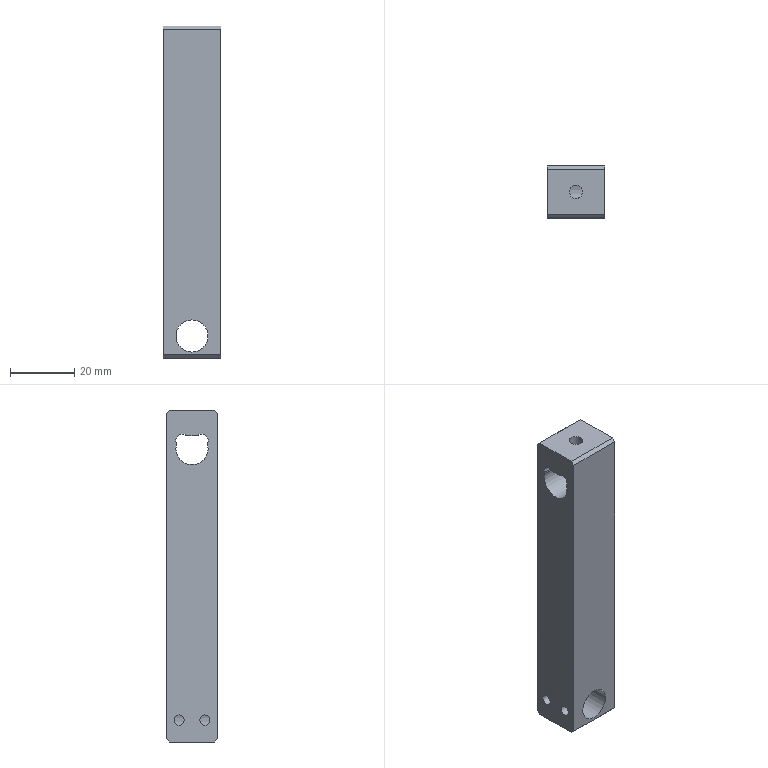NC program | NX | posted by the shop | part box 18 x 16 x 103.264 mm
Whole program:
%
O0001
(Machine time: 45.49 MIN)
(===Total Tool:6===)
(T2=D6 chamfer mill   D=6.   R=0.   D-  H02 Z=-2.15 )
(T13=ZT3.3  D=3.3  DR_a=118 D-  H13 Z=-10.  )
(T16=ZT6.8  D=6.8  DR_a=118 D-  H16 Z=-22.  )
(T4=D4      D=4.   R=0.   D-  H04 Z=-18.5 )
(T21=M4X0.7 D=3.3  DR_a=180 D-  H21 Z=-7.   )
(T11=D4-J   D=4.   R=0.   D11 H11 Z=-18.5 )
G80 G90 G17 G49 G40
G91 G28 Z0
M01
N1 T02 M06
(D6 chamfer mill  D=6. R=0. H=02 ce=0.00 di=0.00)
G00 G90 G54 X96.43 Y-12. M03 S8000
G43 H02 Z20.
M08
G98 G81 X96.43 Y-12. Z-.8 R1. F500.
Y-4.
G80
G00 Z20.
G00 G90 X12. Y-8. M03 S8000
Z20.
G98 G81 X12. Y-8. Z-.8 R1. F500.
G80
G00 Z20.
G91 G28 Z0.0
M05
M09
G91 G28 Z0.0
M01
N2 T13 M06
(ZT3.3 D=3.3 DR_a=118 H=13)
G00 G90 G54 X96.43 Y-12. M03 S3000
G43 H13 Z20.
M08
G98 G83 X96.43 Y-12. Z-10. R1. F300. Q2.
Y-4.
G80
G00 Z20.
G91 G28 Z0.0
M05
M09
G91 G28 Z0.0
M01
N3 T16 M06
(ZT6.8 D=6.8 DR_a=118 H=16)
G00 G90 G54 X12. Y-8. M03 S2000
G43 H16 Z20.
M08
G98 G83 X12. Y-8. Z-22. R1. F300. Q2.
G80
G00 Z20.
G91 G28 Z0.0
M05
M09
G91 G28 Z0.0
M01
N4 T04 M06
(D4  D=4. R=0. H=04 ce=0.05 di=0.10)
G00 G90 G54 X10.02 Y-7.531 M03 S8000
G43 H04 Z20.
M08
Z1.
G01 Y-10.039 Z.869 F2000.
X9.825 Y-10.628 Z.836
X9.615 Y-10.91 Z.818
X10.027 Y-10.789 Z.795
X10.834 Y-10.776 Z.753
X11.659 Y-10.991 Z.708
X12.623 Y-10.945 Z.658
X13.523 Y-10.596 Z.607
X14.266 Y-9.981 Z.556
X14.777 Y-9.162 Z.506
X14.991 Y-8.341 Z.461
X14.945 Y-7.377 Z.411
X14.596 Y-6.477 Z.36
X13.981 Y-5.734 Z.31
X13.162 Y-5.223 Z.259
X12.341 Y-5.009 Z.215
X11.659 Z.179
X10.834 Y-5.224 Z.134
X10.027 Y-5.211 Z.092
X9.615 Y-5.09 Z.069
X9.825 Y-5.372 Z.051
X10.02 Y-5.961 Z.018
Y-6.313 Z0.0
Y-9.687 Z-.05
G02 X9.615 Y-10.91 Z-.069 I-2.05 J0.0
X11.248 Y-10.884 Z-.094 I.864 J-2.925
G03 X14.884 Y-8.752 Z-.163 I.752 J2.884
X12.752 Y-5.116 Z-.232 I-2.884 J.752
X11.248 Y-5.116 Z-.255 I-.752 J-2.884
G02 X9.615 Y-5.09 Z-.279 I-.769 J2.951
X10.02 Y-6.313 Z-.298 I-1.645 J-1.223
G01 Y-9.687 Z-.348
G02 X9.615 Y-10.91 Z-.368 I-2.05 J0.0
X11.248 Y-10.884 Z-.392 I.864 J-2.925
G03 X14.884 Y-8.752 Z-.461 I.752 J2.884
X12.752 Y-5.116 Z-.53 I-2.884 J.752
X11.248 Y-5.116 Z-.553 I-.752 J-2.884
G02 X9.615 Y-5.09 Z-.577 I-.769 J2.951
X10.02 Y-6.313 Z-.597 I-1.645 J-1.223
G01 Y-9.687 Z-.647
G02 X9.615 Y-10.91 Z-.666 I-2.05 J0.0
X11.248 Y-10.884 Z-.69 I.864 J-2.925
G03 X14.884 Y-8.752 Z-.76 I.752 J2.884
X12.752 Y-5.116 Z-.829 I-2.884 J.752
X11.248 Y-5.116 Z-.851 I-.752 J-2.884
G02 X9.615 Y-5.09 Z-.876 I-.769 J2.951
X10.02 Y-6.313 Z-.895 I-1.645 J-1.223
G01 Y-9.687 Z-.945
G02 X9.615 Y-10.91 Z-.964 I-2.05 J0.0
X11.248 Y-10.884 Z-.989 I.864 J-2.925
G03 X14.884 Y-8.752 Z-1.058 I.752 J2.884
X12.752 Y-5.116 Z-1.127 I-2.884 J.752
X11.248 Y-5.116 Z-1.15 I-.752 J-2.884
G02 X9.615 Y-5.09 Z-1.174 I-.769 J2.951
X10.02 Y-6.313 Z-1.194 I-1.645 J-1.223
G01 Y-9.687 Z-1.243
G02 X9.615 Y-10.91 Z-1.263 I-2.05 J0.0
X11.248 Y-10.884 Z-1.287 I.864 J-2.925
G03 X14.884 Y-8.752 Z-1.356 I.752 J2.884
X12.752 Y-5.116 Z-1.426 I-2.884 J.752
X11.248 Y-5.116 Z-1.448 I-.752 J-2.884
G02 X9.615 Y-5.09 Z-1.473 I-.769 J2.951
X10.02 Y-6.313 Z-1.492 I-1.645 J-1.223
G01 Y-9.687 Z-1.542
G02 X9.615 Y-10.91 Z-1.561 I-2.05 J0.0
X11.248 Y-10.884 Z-1.586 I.864 J-2.925
G03 X14.884 Y-8.752 Z-1.655 I.752 J2.884
X12.752 Y-5.116 Z-1.724 I-2.884 J.752
X11.248 Y-5.116 Z-1.747 I-.752 J-2.884
G02 X9.615 Y-5.09 Z-1.771 I-.769 J2.951
X10.02 Y-6.313 Z-1.79 I-1.645 J-1.223
G01 Y-9.687 Z-1.84
G02 X9.615 Y-10.91 Z-1.86 I-2.05 J0.0
X11.248 Y-10.884 Z-1.884 I.864 J-2.925
G03 X14.884 Y-8.752 Z-1.953 I.752 J2.884
X12.752 Y-5.116 Z-2.022 I-2.884 J.752
X11.248 Y-5.116 Z-2.045 I-.752 J-2.884
G02 X9.615 Y-5.09 Z-2.069 I-.769 J2.951
X10.02 Y-6.313 Z-2.089 I-1.645 J-1.223
G01 Y-9.687 Z-2.139
G02 X9.615 Y-10.91 Z-2.158 I-2.05 J0.0
X11.248 Y-10.884 Z-2.182 I.864 J-2.925
G03 X14.884 Y-8.752 Z-2.252 I.752 J2.884
X12.752 Y-5.116 Z-2.321 I-2.884 J.752
X11.248 Y-5.116 Z-2.343 I-.752 J-2.884
G02 X9.615 Y-5.09 Z-2.368 I-.769 J2.951
X10.02 Y-6.313 Z-2.387 I-1.645 J-1.223
G01 Y-9.687 Z-2.437
G02 X9.615 Y-10.91 Z-2.456 I-2.05 J0.0
X11.248 Y-10.884 Z-2.481 I.864 J-2.925
G03 X14.884 Y-8.752 Z-2.55 I.752 J2.884
X12.752 Y-5.116 Z-2.619 I-2.884 J.752
X11.248 Y-5.116 Z-2.642 I-.752 J-2.884
G02 X9.615 Y-5.09 Z-2.666 I-.769 J2.951
X10.02 Y-6.313 Z-2.685 I-1.645 J-1.223
G01 Y-9.687 Z-2.735
G02 X9.615 Y-10.91 Z-2.755 I-2.05 J0.0
X11.248 Y-10.884 Z-2.779 I.864 J-2.925
G03 X14.884 Y-8.752 Z-2.848 I.752 J2.884
X12.752 Y-5.116 Z-2.918 I-2.884 J.752
X11.248 Y-5.116 Z-2.94 I-.752 J-2.884
G02 X9.615 Y-5.09 Z-2.964 I-.769 J2.951
X10.02 Y-6.313 Z-2.984 I-1.645 J-1.223
G01 Y-9.687 Z-3.034
G02 X9.615 Y-10.91 Z-3.053 I-2.05 J0.0
X11.248 Y-10.884 Z-3.078 I.864 J-2.925
G03 X14.884 Y-8.752 Z-3.147 I.752 J2.884
X12.752 Y-5.116 Z-3.216 I-2.884 J.752
X11.248 Y-5.116 Z-3.238 I-.752 J-2.884
G02 X9.615 Y-5.09 Z-3.263 I-.769 J2.951
X10.02 Y-6.313 Z-3.282 I-1.645 J-1.223
G01 Y-9.687 Z-3.332
G02 X9.615 Y-10.91 Z-3.352 I-2.05 J0.0
X11.248 Y-10.884 Z-3.376 I.864 J-2.925
G03 X14.884 Y-8.752 Z-3.445 I.752 J2.884
X12.752 Y-5.116 Z-3.514 I-2.884 J.752
X11.248 Y-5.116 Z-3.537 I-.752 J-2.884
G02 X9.615 Y-5.09 Z-3.561 I-.769 J2.951
X10.02 Y-6.313 Z-3.581 I-1.645 J-1.223
G01 Y-9.687 Z-3.631
G02 X9.615 Y-10.91 Z-3.65 I-2.05 J0.0
X11.248 Y-10.884 Z-3.674 I.864 J-2.925
G03 X14.884 Y-8.752 Z-3.744 I.752 J2.884
X12.752 Y-5.116 Z-3.813 I-2.884 J.752
X11.248 Y-5.116 Z-3.835 I-.752 J-2.884
G02 X9.615 Y-5.09 Z-3.86 I-.769 J2.951
X10.02 Y-6.313 Z-3.879 I-1.645 J-1.223
G01 Y-9.687 Z-3.929
G02 X9.615 Y-10.91 Z-3.948 I-2.05 J0.0
X11.248 Y-10.884 Z-3.973 I.864 J-2.925
G03 X14.884 Y-8.752 Z-4.042 I.752 J2.884
X12.752 Y-5.116 Z-4.111 I-2.884 J.752
X11.248 Y-5.116 Z-4.134 I-.752 J-2.884
G02 X9.615 Y-5.09 Z-4.158 I-.769 J2.951
X10.02 Y-6.313 Z-4.177 I-1.645 J-1.223
G01 Y-9.687 Z-4.227
G02 X9.615 Y-10.91 Z-4.247 I-2.05 J0.0
X11.248 Y-10.884 Z-4.271 I.864 J-2.925
G03 X14.884 Y-8.752 Z-4.34 I.752 J2.884
X12.752 Y-5.116 Z-4.41 I-2.884 J.752
X11.248 Y-5.116 Z-4.432 I-.752 J-2.884
G02 X9.615 Y-5.09 Z-4.456 I-.769 J2.951
X10.02 Y-6.313 Z-4.476 I-1.645 J-1.223
G01 Y-9.687 Z-4.526
G02 X9.615 Y-10.91 Z-4.545 I-2.05 J0.0
X11.248 Y-10.884 Z-4.57 I.864 J-2.925
G03 X14.884 Y-8.752 Z-4.639 I.752 J2.884
X12.752 Y-5.116 Z-4.708 I-2.884 J.752
X11.248 Y-5.116 Z-4.73 I-.752 J-2.884
G02 X9.615 Y-5.09 Z-4.755 I-.769 J2.951
X10.02 Y-6.313 Z-4.774 I-1.645 J-1.223
G01 Y-9.687 Z-4.824
G02 X9.615 Y-10.91 Z-4.843 I-2.05 J0.0
X11.248 Y-10.884 Z-4.868 I.864 J-2.925
G03 X14.884 Y-8.752 Z-4.937 I.752 J2.884
X12.752 Y-5.116 Z-5.006 I-2.884 J.752
X11.248 Y-5.116 Z-5.029 I-.752 J-2.884
G02 X9.615 Y-5.09 Z-5.053 I-.769 J2.951
X10.02 Y-6.313 Z-5.073 I-1.645 J-1.223
G01 Y-9.687 Z-5.122
G02 X9.615 Y-10.91 Z-5.142 I-2.05 J0.0
X11.248 Y-10.884 Z-5.166 I.864 J-2.925
G03 X14.884 Y-8.752 Z-5.235 I.752 J2.884
X12.752 Y-5.116 Z-5.305 I-2.884 J.752
X11.248 Y-5.116 Z-5.327 I-.752 J-2.884
G02 X9.615 Y-5.09 Z-5.352 I-.769 J2.951
X10.02 Y-6.313 Z-5.371 I-1.645 J-1.223
G01 Y-9.687 Z-5.421
G02 X9.615 Y-10.91 Z-5.44 I-2.05 J0.0
X11.248 Y-10.884 Z-5.465 I.864 J-2.925
G03 X14.884 Y-8.752 Z-5.534 I.752 J2.884
X12.752 Y-5.116 Z-5.603 I-2.884 J.752
X11.248 Y-5.116 Z-5.626 I-.752 J-2.884
G02 X9.615 Y-5.09 Z-5.65 I-.769 J2.951
X10.02 Y-6.313 Z-5.669 I-1.645 J-1.223
G01 Y-9.687 Z-5.719
G02 X9.615 Y-10.91 Z-5.739 I-2.05 J0.0
X11.248 Y-10.884 Z-5.763 I.864 J-2.925
G03 X14.884 Y-8.752 Z-5.832 I.752 J2.884
X12.752 Y-5.116 Z-5.901 I-2.884 J.752
X11.248 Y-5.116 Z-5.924 I-.752 J-2.884
G02 X9.615 Y-5.09 Z-5.948 I-.769 J2.951
X10.02 Y-6.313 Z-5.968 I-1.645 J-1.223
G01 Y-9.687 Z-6.018
G02 X9.615 Y-10.91 Z-6.037 I-2.05 J0.0
X11.248 Y-10.884 Z-6.061 I.864 J-2.925
G03 X14.884 Y-8.752 Z-6.131 I.752 J2.884
X12.752 Y-5.116 Z-6.2 I-2.884 J.752
X11.248 Y-5.116 Z-6.222 I-.752 J-2.884
G02 X9.615 Y-5.09 Z-6.247 I-.769 J2.951
X10.02 Y-6.313 Z-6.266 I-1.645 J-1.223
G01 Y-9.687 Z-6.316
G02 X9.615 Y-10.91 Z-6.335 I-2.05 J0.0
X11.248 Y-10.884 Z-6.36 I.864 J-2.925
G03 X14.884 Y-8.752 Z-6.429 I.752 J2.884
X12.752 Y-5.116 Z-6.498 I-2.884 J.752
X11.248 Y-5.116 Z-6.521 I-.752 J-2.884
G02 X9.615 Y-5.09 Z-6.545 I-.769 J2.951
X10.02 Y-6.313 Z-6.565 I-1.645 J-1.223
G01 Y-9.687 Z-6.614
G02 X9.615 Y-10.91 Z-6.634 I-2.05 J0.0
X11.248 Y-10.884 Z-6.658 I.864 J-2.925
G03 X14.884 Y-8.752 Z-6.727 I.752 J2.884
X12.752 Y-5.116 Z-6.797 I-2.884 J.752
X11.248 Y-5.116 Z-6.819 I-.752 J-2.884
G02 X9.615 Y-5.09 Z-6.844 I-.769 J2.951
X10.02 Y-6.313 Z-6.863 I-1.645 J-1.223
G01 Y-9.687 Z-6.913
G02 X9.615 Y-10.91 Z-6.932 I-2.05 J0.0
X11.248 Y-10.884 Z-6.957 I.864 J-2.925
G03 X14.884 Y-8.752 Z-7.026 I.752 J2.884
X12.752 Y-5.116 Z-7.095 I-2.884 J.752
X11.248 Y-5.116 Z-7.117 I-.752 J-2.884
G02 X9.615 Y-5.09 Z-7.142 I-.769 J2.951
X10.02 Y-6.313 Z-7.161 I-1.645 J-1.223
G01 Y-9.687 Z-7.211
G02 X9.615 Y-10.91 Z-7.231 I-2.05 J0.0
X11.248 Y-10.884 Z-7.255 I.864 J-2.925
G03 X14.884 Y-8.752 Z-7.324 I.752 J2.884
X12.752 Y-5.116 Z-7.393 I-2.884 J.752
X11.248 Y-5.116 Z-7.416 I-.752 J-2.884
G02 X9.615 Y-5.09 Z-7.44 I-.769 J2.951
X10.02 Y-6.313 Z-7.46 I-1.645 J-1.223
G01 Y-9.687 Z-7.51
G02 X9.615 Y-10.91 Z-7.529 I-2.05 J0.0
X11.248 Y-10.884 Z-7.553 I.864 J-2.925
G03 X14.884 Y-8.752 Z-7.623 I.752 J2.884
X12.752 Y-5.116 Z-7.692 I-2.884 J.752
X11.248 Y-5.116 Z-7.714 I-.752 J-2.884
G02 X9.615 Y-5.09 Z-7.739 I-.769 J2.951
X10.02 Y-6.313 Z-7.758 I-1.645 J-1.223
G01 Y-9.687 Z-7.808
G02 X9.615 Y-10.91 Z-7.827 I-2.05 J0.0
X11.248 Y-10.884 Z-7.852 I.864 J-2.925
G03 X14.884 Y-8.752 Z-7.921 I.752 J2.884
X12.752 Y-5.116 Z-7.99 I-2.884 J.752
X11.248 Y-5.116 Z-8.013 I-.752 J-2.884
G02 X9.615 Y-5.09 Z-8.037 I-.769 J2.951
X10.02 Y-6.313 Z-8.056 I-1.645 J-1.223
G01 Y-9.687 Z-8.106
G02 X9.615 Y-10.91 Z-8.126 I-2.05 J0.0
X11.248 Y-10.884 Z-8.15 I.864 J-2.925
G03 X14.884 Y-8.752 Z-8.219 I.752 J2.884
X12.752 Y-5.116 Z-8.289 I-2.884 J.752
X11.248 Y-5.116 Z-8.311 I-.752 J-2.884
G02 X9.615 Y-5.09 Z-8.335 I-.769 J2.951
X10.02 Y-6.313 Z-8.355 I-1.645 J-1.223
G01 Y-9.687 Z-8.405
G02 X9.615 Y-10.91 Z-8.424 I-2.05 J0.0
X11.248 Y-10.884 Z-8.449 I.864 J-2.925
G03 X14.884 Y-8.752 Z-8.518 I.752 J2.884
X12.752 Y-5.116 Z-8.587 I-2.884 J.752
X11.248 Y-5.116 Z-8.609 I-.752 J-2.884
G02 X9.615 Y-5.09 Z-8.634 I-.769 J2.951
X10.02 Y-6.313 Z-8.653 I-1.645 J-1.223
G01 Y-9.687 Z-8.703
G02 X9.615 Y-10.91 Z-8.722 I-2.05 J0.0
X11.248 Y-10.884 Z-8.747 I.864 J-2.925
G03 X14.884 Y-8.752 Z-8.816 I.752 J2.884
X12.752 Y-5.116 Z-8.885 I-2.884 J.752
X11.248 Y-5.116 Z-8.908 I-.752 J-2.884
G02 X9.615 Y-5.09 Z-8.932 I-.769 J2.951
X10.02 Y-6.313 Z-8.952 I-1.645 J-1.223
G01 Y-9.687 Z-9.001
G02 X9.615 Y-10.91 Z-9.021 I-2.05 J0.0
X11.248 Y-10.884 Z-9.045 I.864 J-2.925
G03 X14.884 Y-8.752 Z-9.115 I.752 J2.884
X12.752 Y-5.116 Z-9.184 I-2.884 J.752
X11.248 Y-5.116 Z-9.206 I-.752 J-2.884
G02 X9.615 Y-5.09 Z-9.231 I-.769 J2.951
X10.02 Y-6.313 Z-9.25 I-1.645 J-1.223
G01 Y-9.687 Z-9.3
G02 X9.615 Y-10.91 Z-9.319 I-2.05 J0.0
X11.248 Y-10.884 Z-9.344 I.864 J-2.925
G03 X14.884 Y-8.752 Z-9.413 I.752 J2.884
X12.752 Y-5.116 Z-9.482 I-2.884 J.752
X11.248 Y-5.116 Z-9.505 I-.752 J-2.884
G02 X9.615 Y-5.09 Z-9.529 I-.769 J2.951
X10.02 Y-6.313 Z-9.548 I-1.645 J-1.223
G01 Y-9.687 Z-9.598
G02 X9.615 Y-10.91 Z-9.618 I-2.05 J0.0
X11.248 Y-10.884 Z-9.642 I.864 J-2.925
G03 X14.884 Y-8.752 Z-9.711 I.752 J2.884
X12.752 Y-5.116 Z-9.78 I-2.884 J.752
X11.248 Y-5.116 Z-9.803 I-.752 J-2.884
G02 X9.615 Y-5.09 Z-9.827 I-.769 J2.951
X10.02 Y-6.313 Z-9.847 I-1.645 J-1.223
G01 Y-9.687 Z-9.897
G02 X9.615 Y-10.91 Z-9.916 I-2.05 J0.0
X11.248 Y-10.884 Z-9.94 I.864 J-2.925
G03 X14.884 Y-8.752 Z-10.01 I.752 J2.884
X12.752 Y-5.116 Z-10.079 I-2.884 J.752
X11.248 Y-5.116 Z-10.101 I-.752 J-2.884
G02 X9.615 Y-5.09 Z-10.126 I-.769 J2.951
X10.02 Y-6.313 Z-10.145 I-1.645 J-1.223
G01 Y-9.687 Z-10.195
G02 X9.615 Y-10.91 Z-10.214 I-2.05 J0.0
X11.248 Y-10.884 Z-10.239 I.864 J-2.925
G03 X14.884 Y-8.752 Z-10.308 I.752 J2.884
X12.752 Y-5.116 Z-10.377 I-2.884 J.752
X11.248 Y-5.116 Z-10.4 I-.752 J-2.884
G02 X9.615 Y-5.09 Z-10.424 I-.769 J2.951
X10.02 Y-6.313 Z-10.444 I-1.645 J-1.223
G01 Y-9.687 Z-10.493
G02 X9.615 Y-10.91 Z-10.513 I-2.05 J0.0
X11.248 Y-10.884 Z-10.537 I.864 J-2.925
G03 X14.884 Y-8.752 Z-10.606 I.752 J2.884
X12.752 Y-5.116 Z-10.676 I-2.884 J.752
X11.248 Y-5.116 Z-10.698 I-.752 J-2.884
G02 X9.615 Y-5.09 Z-10.723 I-.769 J2.951
X10.02 Y-6.313 Z-10.742 I-1.645 J-1.223
G01 Y-9.687 Z-10.792
G02 X9.615 Y-10.91 Z-10.811 I-2.05 J0.0
X11.248 Y-10.884 Z-10.836 I.864 J-2.925
G03 X14.884 Y-8.752 Z-10.905 I.752 J2.884
X12.752 Y-5.116 Z-10.974 I-2.884 J.752
X11.248 Y-5.116 Z-10.997 I-.752 J-2.884
G02 X9.615 Y-5.09 Z-11.021 I-.769 J2.951
X10.02 Y-6.313 Z-11.04 I-1.645 J-1.223
G01 Y-9.687 Z-11.09
G02 X9.615 Y-10.91 Z-11.11 I-2.05 J0.0
X11.248 Y-10.884 Z-11.134 I.864 J-2.925
G03 X14.884 Y-8.752 Z-11.203 I.752 J2.884
X12.752 Y-5.116 Z-11.272 I-2.884 J.752
X11.248 Y-5.116 Z-11.295 I-.752 J-2.884
G02 X9.615 Y-5.09 Z-11.319 I-.769 J2.951
X10.02 Y-6.313 Z-11.339 I-1.645 J-1.223
G01 Y-9.687 Z-11.389
G02 X9.615 Y-10.91 Z-11.408 I-2.05 J0.0
X11.248 Y-10.884 Z-11.432 I.864 J-2.925
G03 X14.884 Y-8.752 Z-11.502 I.752 J2.884
X12.752 Y-5.116 Z-11.571 I-2.884 J.752
X11.248 Y-5.116 Z-11.593 I-.752 J-2.884
G02 X9.615 Y-5.09 Z-11.618 I-.769 J2.951
X10.02 Y-6.313 Z-11.637 I-1.645 J-1.223
G01 Y-9.687 Z-11.687
G02 X9.615 Y-10.91 Z-11.706 I-2.05 J0.0
X11.248 Y-10.884 Z-11.731 I.864 J-2.925
G03 X14.884 Y-8.752 Z-11.8 I.752 J2.884
X12.752 Y-5.116 Z-11.869 I-2.884 J.752
X11.248 Y-5.116 Z-11.892 I-.752 J-2.884
G02 X9.615 Y-5.09 Z-11.916 I-.769 J2.951
X10.02 Y-6.313 Z-11.935 I-1.645 J-1.223
G01 Y-9.687 Z-11.985
G02 X9.615 Y-10.91 Z-12.005 I-2.05 J0.0
X11.248 Y-10.884 Z-12.029 I.864 J-2.925
G03 X14.884 Y-8.752 Z-12.098 I.752 J2.884
X12.752 Y-5.116 Z-12.168 I-2.884 J.752
X11.248 Y-5.116 Z-12.19 I-.752 J-2.884
G02 X9.615 Y-5.09 Z-12.214 I-.769 J2.951
X10.02 Y-6.313 Z-12.234 I-1.645 J-1.223
G01 Y-9.687 Z-12.284
G02 X9.615 Y-10.91 Z-12.303 I-2.05 J0.0
X11.248 Y-10.884 Z-12.328 I.864 J-2.925
G03 X14.884 Y-8.752 Z-12.397 I.752 J2.884
X12.752 Y-5.116 Z-12.466 I-2.884 J.752
X11.248 Y-5.116 Z-12.488 I-.752 J-2.884
G02 X9.615 Y-5.09 Z-12.513 I-.769 J2.951
X10.02 Y-6.313 Z-12.532 I-1.645 J-1.223
G01 Y-9.687 Z-12.582
G02 X9.615 Y-10.91 Z-12.602 I-2.05 J0.0
X11.248 Y-10.884 Z-12.626 I.864 J-2.925
G03 X14.884 Y-8.752 Z-12.695 I.752 J2.884
X12.752 Y-5.116 Z-12.764 I-2.884 J.752
X11.248 Y-5.116 Z-12.787 I-.752 J-2.884
G02 X9.615 Y-5.09 Z-12.811 I-.769 J2.951
X10.02 Y-6.313 Z-12.831 I-1.645 J-1.223
G01 Y-9.687 Z-12.881
G02 X9.615 Y-10.91 Z-12.9 I-2.05 J0.0
X11.248 Y-10.884 Z-12.924 I.864 J-2.925
G03 X14.884 Y-8.752 Z-12.994 I.752 J2.884
X12.752 Y-5.116 Z-13.063 I-2.884 J.752
X11.248 Y-5.116 Z-13.085 I-.752 J-2.884
G02 X9.615 Y-5.09 Z-13.11 I-.769 J2.951
X10.02 Y-6.313 Z-13.129 I-1.645 J-1.223
G01 Y-9.687 Z-13.179
G02 X9.615 Y-10.91 Z-13.198 I-2.05 J0.0
X11.248 Y-10.884 Z-13.223 I.864 J-2.925
G03 X14.884 Y-8.752 Z-13.292 I.752 J2.884
X12.752 Y-5.116 Z-13.361 I-2.884 J.752
X11.248 Y-5.116 Z-13.384 I-.752 J-2.884
G02 X9.615 Y-5.09 Z-13.408 I-.769 J2.951
X10.02 Y-6.313 Z-13.427 I-1.645 J-1.223
G01 Y-9.687 Z-13.477
G02 X9.615 Y-10.91 Z-13.497 I-2.05 J0.0
X11.248 Y-10.884 Z-13.521 I.864 J-2.925
G03 X14.884 Y-8.752 Z-13.59 I.752 J2.884
X12.752 Y-5.116 Z-13.66 I-2.884 J.752
X11.248 Y-5.116 Z-13.682 I-.752 J-2.884
G02 X9.615 Y-5.09 Z-13.706 I-.769 J2.951
X10.02 Y-6.313 Z-13.726 I-1.645 J-1.223
G01 Y-9.687 Z-13.776
G02 X9.615 Y-10.91 Z-13.795 I-2.05 J0.0
X11.248 Y-10.884 Z-13.82 I.864 J-2.925
G03 X14.884 Y-8.752 Z-13.889 I.752 J2.884
X12.752 Y-5.116 Z-13.958 I-2.884 J.752
X11.248 Y-5.116 Z-13.98 I-.752 J-2.884
G02 X9.615 Y-5.09 Z-14.005 I-.769 J2.951
X10.02 Y-6.313 Z-14.024 I-1.645 J-1.223
G01 Y-9.687 Z-14.074
G02 X9.615 Y-10.91 Z-14.093 I-2.05 J0.0
X11.248 Y-10.884 Z-14.118 I.864 J-2.925
G03 X14.884 Y-8.752 Z-14.187 I.752 J2.884
X12.752 Y-5.116 Z-14.256 I-2.884 J.752
X11.248 Y-5.116 Z-14.279 I-.752 J-2.884
G02 X9.615 Y-5.09 Z-14.303 I-.769 J2.951
X10.02 Y-6.313 Z-14.323 I-1.645 J-1.223
G01 Y-9.687 Z-14.372
G02 X9.615 Y-10.91 Z-14.392 I-2.05 J0.0
X11.248 Y-10.884 Z-14.416 I.864 J-2.925
G03 X14.884 Y-8.752 Z-14.485 I.752 J2.884
X12.752 Y-5.116 Z-14.555 I-2.884 J.752
X11.248 Y-5.116 Z-14.577 I-.752 J-2.884
G02 X9.615 Y-5.09 Z-14.602 I-.769 J2.951
X10.02 Y-6.313 Z-14.621 I-1.645 J-1.223
G01 Y-9.687 Z-14.671
G02 X9.615 Y-10.91 Z-14.69 I-2.05 J0.0
X11.248 Y-10.884 Z-14.715 I.864 J-2.925
G03 X14.884 Y-8.752 Z-14.784 I.752 J2.884
X12.752 Y-5.116 Z-14.853 I-2.884 J.752
X11.248 Y-5.116 Z-14.876 I-.752 J-2.884
G02 X9.615 Y-5.09 Z-14.9 I-.769 J2.951
X10.02 Y-6.313 Z-14.919 I-1.645 J-1.223
G01 Y-9.687 Z-14.969
G02 X9.615 Y-10.91 Z-14.989 I-2.05 J0.0
X11.248 Y-10.884 Z-15.013 I.864 J-2.925
G03 X14.884 Y-8.752 Z-15.082 I.752 J2.884
X12.752 Y-5.116 Z-15.151 I-2.884 J.752
X11.248 Y-5.116 Z-15.174 I-.752 J-2.884
G02 X9.615 Y-5.09 Z-15.198 I-.769 J2.951
X10.02 Y-6.313 Z-15.218 I-1.645 J-1.223
G01 Y-9.687 Z-15.268
G02 X9.615 Y-10.91 Z-15.287 I-2.05 J0.0
X11.248 Y-10.884 Z-15.311 I.864 J-2.925
G03 X14.884 Y-8.752 Z-15.381 I.752 J2.884
X12.752 Y-5.116 Z-15.45 I-2.884 J.752
X11.248 Y-5.116 Z-15.472 I-.752 J-2.884
G02 X9.615 Y-5.09 Z-15.497 I-.769 J2.951
X10.02 Y-6.313 Z-15.516 I-1.645 J-1.223
G01 Y-9.687 Z-15.566
G02 X9.615 Y-10.91 Z-15.585 I-2.05 J0.0
X11.248 Y-10.884 Z-15.61 I.864 J-2.925
G03 X14.884 Y-8.752 Z-15.679 I.752 J2.884
X12.752 Y-5.116 Z-15.748 I-2.884 J.752
X11.248 Y-5.116 Z-15.771 I-.752 J-2.884
G02 X9.615 Y-5.09 Z-15.795 I-.769 J2.951
X10.02 Y-6.313 Z-15.815 I-1.645 J-1.223
G01 Y-9.687 Z-15.864
G02 X9.615 Y-10.91 Z-15.884 I-2.05 J0.0
X11.248 Y-10.884 Z-15.908 I.864 J-2.925
G03 X14.884 Y-8.752 Z-15.977 I.752 J2.884
X12.752 Y-5.116 Z-16.047 I-2.884 J.752
X11.248 Y-5.116 Z-16.069 I-.752 J-2.884
G02 X9.615 Y-5.09 Z-16.094 I-.769 J2.951
X10.02 Y-6.313 Z-16.113 I-1.645 J-1.223
G01 Y-9.687 Z-16.163
G02 X9.615 Y-10.91 Z-16.182 I-2.05 J0.0
X11.248 Y-10.884 Z-16.207 I.864 J-2.925
G03 X14.884 Y-8.752 Z-16.276 I.752 J2.884
X12.752 Y-5.116 Z-16.345 I-2.884 J.752
X11.248 Y-5.116 Z-16.367 I-.752 J-2.884
G02 X9.615 Y-5.09 Z-16.392 I-.769 J2.951
X10.02 Y-6.313 Z-16.411 I-1.645 J-1.223
G01 Y-9.687 Z-16.461
G02 X9.615 Y-10.91 Z-16.481 I-2.05 J0.0
X11.248 Y-10.884 Z-16.505 I.864 J-2.925
G03 X14.884 Y-8.752 Z-16.574 I.752 J2.884
X12.752 Y-5.116 Z-16.643 I-2.884 J.752
X11.248 Y-5.116 Z-16.666 I-.752 J-2.884
G02 X9.615 Y-5.09 Z-16.69 I-.769 J2.951
X10.02 Y-6.313 Z-16.71 I-1.645 J-1.223
G01 Y-9.687 Z-16.76
G02 X9.615 Y-10.91 Z-16.779 I-2.05 J0.0
X11.248 Y-10.884 Z-16.803 I.864 J-2.925
G03 X14.884 Y-8.752 Z-16.873 I.752 J2.884
X12.752 Y-5.116 Z-16.942 I-2.884 J.752
X11.248 Y-5.116 Z-16.964 I-.752 J-2.884
G02 X9.615 Y-5.09 Z-16.989 I-.769 J2.951
X10.02 Y-6.313 Z-17.008 I-1.645 J-1.223
G01 Y-9.687 Z-17.058
G02 X9.615 Y-10.91 Z-17.077 I-2.05 J0.0
X11.248 Y-10.884 Z-17.102 I.864 J-2.925
G03 X14.884 Y-8.752 Z-17.171 I.752 J2.884
X12.752 Y-5.116 Z-17.24 I-2.884 J.752
X11.248 Y-5.116 Z-17.263 I-.752 J-2.884
G02 X9.615 Y-5.09 Z-17.287 I-.769 J2.951
X10.02 Y-6.313 Z-17.306 I-1.645 J-1.223
G01 Y-9.687 Z-17.356
G02 X9.615 Y-10.91 Z-17.376 I-2.05 J0.0
X11.248 Y-10.884 Z-17.4 I.864 J-2.925
G03 X14.884 Y-8.752 Z-17.469 I.752 J2.884
X12.752 Y-5.116 Z-17.539 I-2.884 J.752
X11.248 Y-5.116 Z-17.561 I-.752 J-2.884
G02 X9.615 Y-5.09 Z-17.585 I-.769 J2.951
X10.02 Y-6.313 Z-17.605 I-1.645 J-1.223
G01 Y-9.687 Z-17.655
G02 X9.615 Y-10.91 Z-17.674 I-2.05 J0.0
X11.248 Y-10.884 Z-17.699 I.864 J-2.925
G03 X14.884 Y-8.752 Z-17.768 I.752 J2.884
X12.752 Y-5.116 Z-17.837 I-2.884 J.752
X11.248 Y-5.116 Z-17.859 I-.752 J-2.884
G02 X9.615 Y-5.09 Z-17.884 I-.769 J2.951
X10.02 Y-6.313 Z-17.903 I-1.645 J-1.223
G01 Y-9.687 Z-17.953
G02 X9.615 Y-10.91 Z-17.972 I-2.05 J0.0
X11.248 Y-10.884 Z-17.997 I.864 J-2.925
G03 X14.884 Y-8.752 Z-18.066 I.752 J2.884
X12.752 Y-5.116 Z-18.135 I-2.884 J.752
X11.248 Y-5.116 Z-18.158 I-.752 J-2.884
G02 X9.615 Y-5.09 Z-18.182 I-.769 J2.951
X10.02 Y-6.313 Z-18.202 I-1.645 J-1.223
G01 Y-9.687 Z-18.251
G02 X9.615 Y-10.91 Z-18.271 I-2.05 J0.0
X11.248 Y-10.884 Z-18.295 I.864 J-2.925
G03 X14.884 Y-8.752 Z-18.365 I.752 J2.884
X12.752 Y-5.116 Z-18.434 I-2.884 J.752
X11.248 Y-5.116 Z-18.456 I-.752 J-2.884
G02 X9.615 Y-5.09 Z-18.481 I-.769 J2.951
X10.02 Y-6.313 Z-18.5 I-1.645 J-1.223
G01 Y-9.687
G02 X9.615 Y-10.91 I-2.05 J0.0
X10.479 Y-10.785 I.864 J-2.925
X11.248 Y-10.884 I0.0 J-3.05
G03 X12. Y-10.98 I.752 J2.884
X14.98 Y-8. I0.0 J2.98
X12. Y-5.02 I-2.98 J0.0
X11.248 Y-5.116 I0.0 J-2.98
G02 X10.479 Y-5.215 I-.769 J2.951
X9.615 Y-5.09 I0.0 J3.05
X10.02 Y-6.313 I-1.645 J-1.223
G01 Y-6.713
Z-17.5
G00 Z20.
G91 G28 Z0.0
M05
M09
G91 G28 Z0.0
M01
N5 T02 M06
(D6 chamfer mill  D=6. R=0. H=02 ce=0.00 di=0.10)
G00 G90 G54 X96.43 Y-12. M03 S8000
G43 H02 Z20.
M08
G98 G81 X96.43 Y-12. Z-2.15 R3. F500.
Y-4.
G80
G00 Z20.
G00 G90 X12.3 Y-3.681 M03 S7000
Z20.
Z2.5
G01 X11.949 Y-3.667 Z2.372 F1500.
X11.504 Y-3.695 Z2.21
X11.064 Y-3.769 Z2.047
X10.81 Y-3.835 Z1.952
X10.54 Y-3.867 Z1.853
X10.269 Y-3.855 Z1.754
X10.003 Y-3.8 Z1.655
X9.824 Y-3.736 Z1.586
X9.583 Y-3.692 Z1.497
X9.338 Y-3.694 Z1.408
X9.097 Y-3.741 Z1.319
X8.87 Y-3.833 Z1.229
X8.664 Y-3.966 Z1.14
X8.486 Y-4.136 Z1.051
X8.344 Y-4.335 Z.962
X8.241 Y-4.558 Z.872
X8.182 Y-4.796 Z.783
X8.168 Y-5.04 Z.694
X8.2 Y-5.283 Z.605
X8.278 Y-5.516 Z.515
X8.398 Y-5.73 Z.426
X8.501 Y-5.86 Z.366
X8.585 Y-6.011 Z.303
X8.642 Y-6.174 Z.24
X8.67 Y-6.344 Z.177
Y-9.578 Z-1.
G02 X8.453 Y-10.201 I-1. J0.0
G03 X8.17 Y-11.01 I1.017 J-.809
X9.47 Y-12.31 I1.3 J0.0
X9.907 Y-12.234 I0.0 J1.3
G02 X10.479 Y-12.135 I.572 J-1.601
X10.908 Y-12.19 I0.0 J-1.7
G03 X12. Y-12.33 I1.092 J4.19
X16.33 Y-8. I0.0 J4.33
X12. Y-3.67 I-4.33 J0.0
X10.908 Y-3.81 I0.0 J-4.33
G02 X10.479 Y-3.865 I-.429 J1.645
X9.907 Y-3.766 I0.0 J1.7
G03 X9.47 Y-3.69 I-.437 J-1.224
X8.17 Y-4.99 I0.0 J-1.3
X8.453 Y-5.799 I1.3 J0.0
G02 X8.67 Y-6.422 I-.783 J-.623
G01 Y-9.578
G02 X8.548 Y-10.058 I-1. J0.0
G01 Z1.5
G00 Z20.
G91 G28 Z0.0
M05
M09
G91 G28 Z0.0
M01
N6 T21 M06
(M4X0.7 D=3.3 DR_a=180 H=21)
G00 G90 G54 X96.43 Y-12. M03 S600
G43 H21 Z20.
M08
G95
G98 G84 X96.43 Y-12. Z-7. R1. F.7 Q4.
Y-4.
G80
G94
G00 Z20.
G91 G28 Z0.0
M05
M09
G91 G28 Z0.0
M01
N7 T11 M06
(D4-J  D=4. R=0. H=11 ce=-0.01 di=0.00)
G00 G90 G54 X14.941 Y-8.769 M03 S8000
G43 H11 Z20.
M08
Z.5
G01 X14.985 Y-8.598 Z.491 F800.
X15.042 Y-8.109 Z.465
X15.02 Y-7.618 Z.439
X14.919 Y-7.136 Z.413
X14.742 Y-6.677 Z.388
X14.493 Y-6.253 Z.362
X14.179 Y-5.874 Z.336
X13.808 Y-5.551 Z.31
X13.39 Y-5.291 Z.284
X12.935 Y-5.103 Z.259
X12.598 Y-5.015 Z.24
X12.2 Y-4.962 Z.219
X11.8 Z.198
X11.402 Y-5.015 Z.177
X11.066 Y-5.102 Z.159
X10.588 Y-5.159 Z.134
X10.107 Y-5.137 Z.109
X9.636 Y-5.039 Z.083
X9.464 Y-4.978 Z.074
X9.459 Y-4.992 Z.073
X9.556 Y-5.102 Z.065
X9.752 Y-5.415 Z.046
X9.887 Y-5.759 Z.027
X9.956 Y-6.122 Z.007
X9.96 Y-6.263 Z0.0
G41 D11
Y-6.313
Y-9.687 Z-.298
G02 X9.463 Y-11.003 Z-.424 I-1.99 J0.0
G01 X9.455 Y-11.011 Z-.425
X9.463 Y-11.017 Z-.426
X9.467 Y-11.025
X9.473 Y-11.019 Z-.427
G02 X11.233 Y-10.942 Z-.584 I1.006 J-2.816
G03 X14.942 Y-8.767 Z-1.005 I.767 J2.942
X12.767 Y-5.058 Z-1.426 I-2.942 J.767
X11.233 Y-5.058 Z-1.563 I-.767 J-2.942
G02 X9.473 Y-4.981 Z-1.721 I-.754 J2.893
G01 X9.464 Y-4.976 Z-1.722
X9.461 Y-4.987
X9.455 Y-4.993 Z-1.723
X9.463 Y-4.997
G02 X9.96 Y-6.313 Z-1.85 I-1.493 J-1.316
G01 Y-9.687 Z-2.148
G02 X9.463 Y-11.003 Z-2.274 I-1.99 J0.0
G01 X9.455 Y-11.011 Z-2.275
X9.463 Y-11.017 Z-2.276
X9.467 Y-11.025
X9.473 Y-11.019 Z-2.277
G02 X11.233 Y-10.942 Z-2.434 I1.006 J-2.816
G03 X14.942 Y-8.767 Z-2.855 I.767 J2.942
X12.767 Y-5.058 Z-3.276 I-2.942 J.767
X11.233 Y-5.058 Z-3.413 I-.767 J-2.942
G02 X9.473 Y-4.981 Z-3.571 I-.754 J2.893
G01 X9.464 Y-4.976 Z-3.572
X9.461 Y-4.987
X9.455 Y-4.993 Z-3.573
X9.463 Y-4.997
G02 X9.96 Y-6.313 Z-3.7 I-1.493 J-1.316
G01 Y-9.687 Z-3.998
G02 X9.463 Y-11.003 Z-4.124 I-1.99 J0.0
G01 X9.455 Y-11.011 Z-4.125
X9.463 Y-11.017 Z-4.126
X9.467 Y-11.025
X9.473 Y-11.019 Z-4.127
G02 X11.233 Y-10.942 Z-4.284 I1.006 J-2.816
G03 X14.942 Y-8.767 Z-4.705 I.767 J2.942
X12.767 Y-5.058 Z-5.126 I-2.942 J.767
X11.233 Y-5.058 Z-5.263 I-.767 J-2.942
G02 X9.473 Y-4.981 Z-5.421 I-.754 J2.893
G01 X9.464 Y-4.976 Z-5.422
X9.461 Y-4.987
X9.455 Y-4.993 Z-5.423
X9.463 Y-4.997
G02 X9.96 Y-6.313 Z-5.55 I-1.493 J-1.316
G01 Y-9.687 Z-5.848
G02 X9.463 Y-11.003 Z-5.974 I-1.99 J0.0
G01 X9.455 Y-11.011 Z-5.975
X9.463 Y-11.017 Z-5.976
X9.467 Y-11.025
X9.473 Y-11.019 Z-5.977
G02 X11.233 Y-10.942 Z-6.134 I1.006 J-2.816
G03 X14.942 Y-8.767 Z-6.555 I.767 J2.942
X12.767 Y-5.058 Z-6.976 I-2.942 J.767
X11.233 Y-5.058 Z-7.113 I-.767 J-2.942
G02 X9.473 Y-4.981 Z-7.271 I-.754 J2.893
G01 X9.464 Y-4.976 Z-7.272
X9.461 Y-4.987
X9.455 Y-4.993 Z-7.273
X9.463 Y-4.997
G02 X9.96 Y-6.313 Z-7.4 I-1.493 J-1.316
G01 Y-9.687 Z-7.698
G02 X9.463 Y-11.003 Z-7.824 I-1.99 J0.0
G01 X9.455 Y-11.011 Z-7.825
X9.463 Y-11.017 Z-7.826
X9.467 Y-11.025
X9.473 Y-11.019 Z-7.827
G02 X11.233 Y-10.942 Z-7.984 I1.006 J-2.816
G03 X14.942 Y-8.767 Z-8.405 I.767 J2.942
X12.767 Y-5.058 Z-8.826 I-2.942 J.767
X11.233 Y-5.058 Z-8.963 I-.767 J-2.942
G02 X9.473 Y-4.981 Z-9.121 I-.754 J2.893
G01 X9.464 Y-4.976 Z-9.122
X9.461 Y-4.987
X9.455 Y-4.993 Z-9.123
X9.463 Y-4.997
G02 X9.96 Y-6.313 Z-9.25 I-1.493 J-1.316
G01 Y-9.687 Z-9.548
G02 X9.463 Y-11.003 Z-9.674 I-1.99 J0.0
G01 X9.455 Y-11.011 Z-9.675
X9.463 Y-11.017 Z-9.676
X9.467 Y-11.025
X9.473 Y-11.019 Z-9.677
G02 X11.233 Y-10.942 Z-9.834 I1.006 J-2.816
G03 X14.942 Y-8.767 Z-10.255 I.767 J2.942
X12.767 Y-5.058 Z-10.676 I-2.942 J.767
X11.233 Y-5.058 Z-10.813 I-.767 J-2.942
G02 X9.473 Y-4.981 Z-10.971 I-.754 J2.893
G01 X9.464 Y-4.976 Z-10.972
X9.461 Y-4.987
X9.455 Y-4.993 Z-10.973
X9.463 Y-4.997
G02 X9.96 Y-6.313 Z-11.1 I-1.493 J-1.316
G01 Y-9.687 Z-11.398
G02 X9.463 Y-11.003 Z-11.524 I-1.99 J0.0
G01 X9.455 Y-11.011 Z-11.525
X9.463 Y-11.017 Z-11.526
X9.467 Y-11.025
X9.473 Y-11.019 Z-11.527
G02 X11.233 Y-10.942 Z-11.684 I1.006 J-2.816
G03 X14.942 Y-8.767 Z-12.105 I.767 J2.942
X12.767 Y-5.058 Z-12.526 I-2.942 J.767
X11.233 Y-5.058 Z-12.663 I-.767 J-2.942
G02 X9.473 Y-4.981 Z-12.821 I-.754 J2.893
G01 X9.464 Y-4.976 Z-12.822
X9.461 Y-4.987
X9.455 Y-4.993 Z-12.823
X9.463 Y-4.997
G02 X9.96 Y-6.313 Z-12.95 I-1.493 J-1.316
G01 Y-9.687 Z-13.248
G02 X9.463 Y-11.003 Z-13.374 I-1.99 J0.0
G01 X9.455 Y-11.011 Z-13.375
X9.463 Y-11.017 Z-13.376
X9.467 Y-11.025
X9.473 Y-11.019 Z-13.377
G02 X11.233 Y-10.942 Z-13.534 I1.006 J-2.816
G03 X14.942 Y-8.767 Z-13.955 I.767 J2.942
X12.767 Y-5.058 Z-14.376 I-2.942 J.767
X11.233 Y-5.058 Z-14.513 I-.767 J-2.942
G02 X9.473 Y-4.981 Z-14.671 I-.754 J2.893
G01 X9.464 Y-4.976 Z-14.672
X9.461 Y-4.987
X9.455 Y-4.993 Z-14.673
X9.463 Y-4.997
G02 X9.96 Y-6.313 Z-14.8 I-1.493 J-1.316
G01 Y-9.687 Z-15.098
G02 X9.463 Y-11.003 Z-15.224 I-1.99 J0.0
G01 X9.455 Y-11.011 Z-15.225
X9.463 Y-11.017 Z-15.226
X9.467 Y-11.025
X9.473 Y-11.019 Z-15.227
G02 X11.233 Y-10.942 Z-15.384 I1.006 J-2.816
G03 X14.942 Y-8.767 Z-15.805 I.767 J2.942
X12.767 Y-5.058 Z-16.226 I-2.942 J.767
X11.233 Y-5.058 Z-16.363 I-.767 J-2.942
G02 X9.473 Y-4.981 Z-16.521 I-.754 J2.893
G01 X9.464 Y-4.976 Z-16.522
X9.461 Y-4.987
X9.455 Y-4.993 Z-16.523
X9.463 Y-4.997
G02 X9.96 Y-6.313 Z-16.65 I-1.493 J-1.316
G01 Y-9.687 Z-16.948
G02 X9.463 Y-11.003 Z-17.074 I-1.99 J0.0
G01 X9.455 Y-11.011 Z-17.075
X9.463 Y-11.017 Z-17.076
X9.467 Y-11.025
X9.473 Y-11.019 Z-17.077
G02 X11.233 Y-10.942 Z-17.234 I1.006 J-2.816
G03 X14.942 Y-8.767 Z-17.655 I.767 J2.942
X12.767 Y-5.058 Z-18.076 I-2.942 J.767
X11.233 Y-5.058 Z-18.213 I-.767 J-2.942
G02 X9.473 Y-4.981 Z-18.371 I-.754 J2.893
G01 X9.464 Y-4.976 Z-18.372
X9.461 Y-4.987
X9.455 Y-4.993 Z-18.373
X9.463 Y-4.997
G02 X9.96 Y-6.313 Z-18.5 I-1.493 J-1.316
G01 Y-9.687
G02 X9.463 Y-11.003 I-1.99 J0.0
G01 X9.455 Y-11.012
X9.462 Y-11.023
X9.473 Y-11.019
G02 X10.479 Y-10.845 I1.006 J-2.816
X11.233 Y-10.942 I0.0 J-2.99
G03 X12. Y-11.04 I.767 J2.942
X15.04 Y-8. I0.0 J3.04
X12. Y-4.96 I-3.04 J0.0
X11.233 Y-5.058 I0.0 J-3.04
G02 X10.479 Y-5.155 I-.754 J2.893
X9.473 Y-4.981 I0.0 J2.99
G01 X9.462 Y-4.977
X9.455 Y-4.988
X9.463 Y-4.997
G02 X9.96 Y-6.313 I-1.493 J-1.316
G01 Y-6.713
X9.962 Y-6.74
X9.983 Y-6.761
X10.01 Y-6.763
G40 X10.06
Z-17.5
G00 Z20.
M05
M09
G91 G28 Z0.0
G91 G28 Y0.0
M30
%